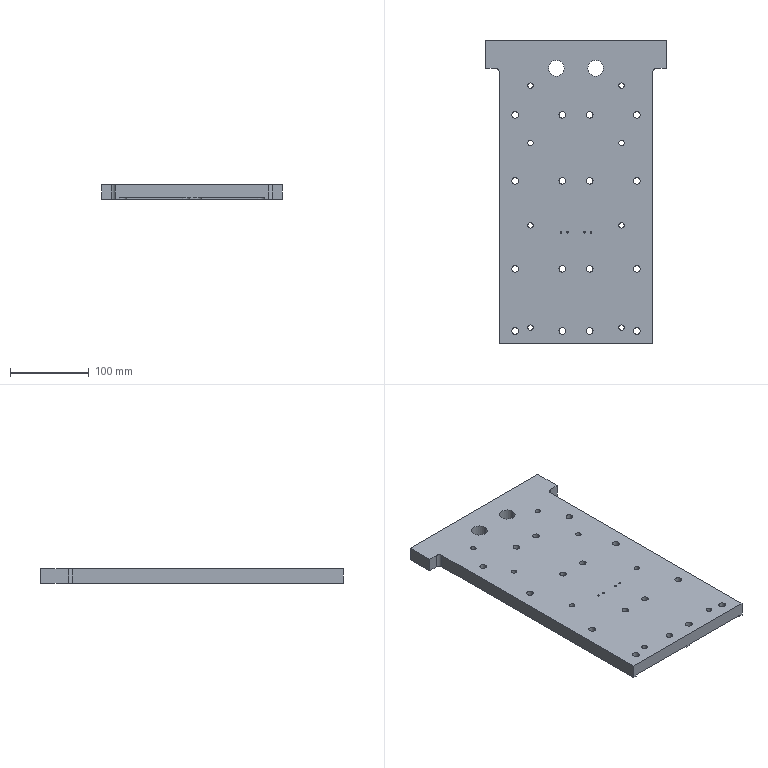Part | 1 solid | 112 faces | box 230 x 385 x 18 mm | volume 1218322 mm3 | cylinder 76 | plane 18 | cone 18 | commonest cylinder face diameters 8.5 x32 6.8 x26 2.5 x8 10 x6 20 x4